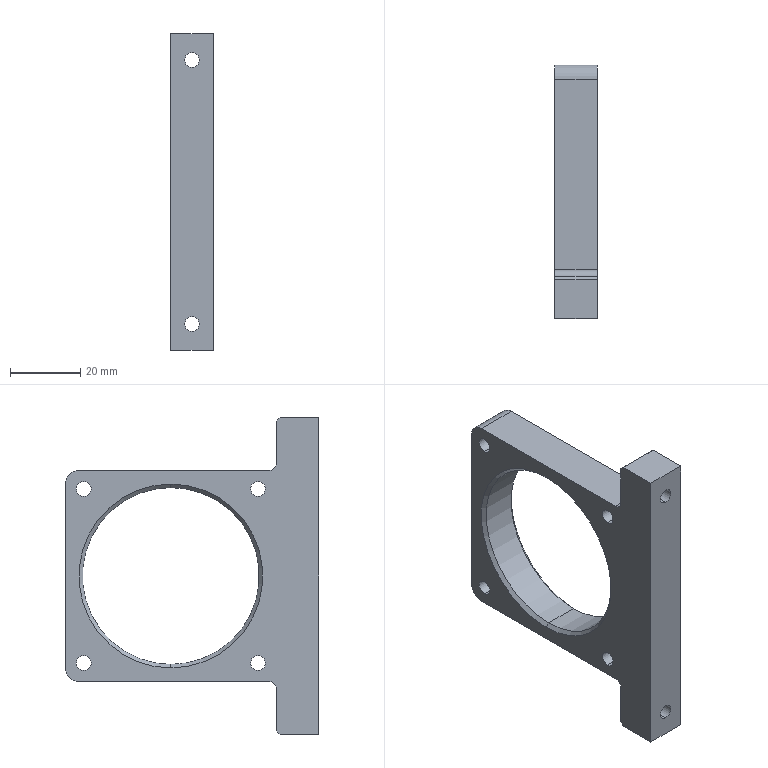Part | SolidWorks | features Chamfer 2, Fillet 2, HoleWzd 2, Extrusion 1 | 1 solid | 34 faces | box 12 x 72 x 90 mm | volume 31178 mm3 | cylinder 18 | plane 12 | cone 4 | commonest cylinder face diameters 4.2 x12 4 x2 8 x2 50.2 x2
STEP:
#1=CARTESIAN_POINT('',(5.,42.,25.1));
#2=VERTEX_POINT('',#1);
#3=CARTESIAN_POINT('',(5.,42.,-25.1));
#4=VERTEX_POINT('',#3);
#5=CARTESIAN_POINT('',(5.,42.,0.));
#6=DIRECTION('',(1.,0.,0.));
#7=DIRECTION('',(0.,0.,1.));
#8=AXIS2_PLACEMENT_3D('',#5,#6,#7);
#9=CIRCLE('',#8,25.1);
#10=EDGE_CURVE('',#2,#4,#9,.T.);
#11=ORIENTED_EDGE('',*,*,#10,.F.);
#12=CARTESIAN_POINT('',(6.,42.,26.1));
#13=VERTEX_POINT('',#12);
#14=CARTESIAN_POINT('',(5.,42.,25.1));
#15=DIRECTION('',(0.7071,0.,0.7071));
#16=VECTOR('',#15,1000.);
#17=LINE('',#14,#16);
#18=EDGE_CURVE('',#2,#13,#17,.T.);
#19=ORIENTED_EDGE('',*,*,#18,.T.);
#20=CARTESIAN_POINT('',(6.,42.,-26.1));
#21=VERTEX_POINT('',#20);
#22=CARTESIAN_POINT('',(6.,42.,0.));
#23=DIRECTION('',(-1.,0.,0.));
#24=DIRECTION('',(0.,0.,1.));
#25=AXIS2_PLACEMENT_3D('',#22,#23,#24);
#26=CIRCLE('',#25,26.1);
#27=EDGE_CURVE('',#21,#13,#26,.T.);
#28=ORIENTED_EDGE('',*,*,#27,.F.);
#29=CARTESIAN_POINT('',(5.,42.,-25.1));
#30=DIRECTION('',(0.7071,0.,-0.7071));
#31=VECTOR('',#30,1000.);
#32=LINE('',#29,#31);
#33=EDGE_CURVE('',#4,#21,#32,.T.);
#34=ORIENTED_EDGE('',*,*,#33,.F.);
#35=EDGE_LOOP('',(#11,#19,#28,#34));
#36=FACE_OUTER_BOUND('',#35,.T.);
#37=CARTESIAN_POINT('',(5.,42.,0.));
#38=DIRECTION('',(1.,0.,0.));
#39=DIRECTION('',(0.,0.,-1.));
#40=AXIS2_PLACEMENT_3D('',#37,#38,#39);
#41=CONICAL_SURFACE('',#40,25.1,0.7854);
#42=ADVANCED_FACE('',(#36),#41,.F.);
#43=CARTESIAN_POINT('',(-5.,42.,-25.1));
#44=VERTEX_POINT('',#43);
#45=CARTESIAN_POINT('',(-5.,42.,25.1));
#46=VERTEX_POINT('',#45);
#47=CARTESIAN_POINT('',(-5.,42.,0.));
#48=DIRECTION('',(-1.,0.,0.));
#49=DIRECTION('',(0.,0.,1.));
#50=AXIS2_PLACEMENT_3D('',#47,#48,#49);
#51=CIRCLE('',#50,25.1);
#52=EDGE_CURVE('',#44,#46,#51,.T.);
#53=ORIENTED_EDGE('',*,*,#52,.F.);
#54=CARTESIAN_POINT('',(-6.,42.,-26.1));
#55=VERTEX_POINT('',#54);
#56=CARTESIAN_POINT('',(-6.,42.,-26.1));
#57=DIRECTION('',(-0.7071,0.,-0.7071));
#58=VECTOR('',#57,1000.);
#59=LINE('',#56,#58);
#60=EDGE_CURVE('',#44,#55,#59,.T.);
#61=ORIENTED_EDGE('',*,*,#60,.T.);
#62=CARTESIAN_POINT('',(-6.,42.,26.1));
#63=VERTEX_POINT('',#62);
#64=CARTESIAN_POINT('',(-6.,42.,0.));
#65=DIRECTION('',(1.,0.,0.));
#66=DIRECTION('',(0.,0.,1.));
#67=AXIS2_PLACEMENT_3D('',#64,#65,#66);
#68=CIRCLE('',#67,26.1);
#69=EDGE_CURVE('',#63,#55,#68,.T.);
#70=ORIENTED_EDGE('',*,*,#69,.F.);
#71=CARTESIAN_POINT('',(-6.,42.,26.1));
#72=DIRECTION('',(-0.7071,0.,0.7071));
#73=VECTOR('',#72,1000.);
#74=LINE('',#71,#73);
#75=EDGE_CURVE('',#46,#63,#74,.T.);
#76=ORIENTED_EDGE('',*,*,#75,.F.);
#77=EDGE_LOOP('',(#53,#61,#70,#76));
#78=FACE_OUTER_BOUND('',#77,.T.);
#79=CARTESIAN_POINT('',(-6.,42.,0.));
#80=DIRECTION('',(-1.,0.,0.));
#81=DIRECTION('',(0.,0.,1.));
#82=AXIS2_PLACEMENT_3D('',#79,#80,#81);
#83=CONICAL_SURFACE('',#82,26.1,0.7854);
#84=ADVANCED_FACE('',(#78),#83,.F.);
#85=CARTESIAN_POINT('',(-6.,66.749,22.649));
#86=VERTEX_POINT('',#85);
#87=CARTESIAN_POINT('',(-6.,66.749,26.849));
#88=VERTEX_POINT('',#87);
#89=CARTESIAN_POINT('',(-6.,66.749,24.749));
#90=DIRECTION('',(-1.,0.,0.));
#91=DIRECTION('',(0.,0.,1.));
#92=AXIS2_PLACEMENT_3D('',#89,#90,#91);
#93=CIRCLE('',#92,2.1);
#94=EDGE_CURVE('',#86,#88,#93,.T.);
#95=ORIENTED_EDGE('',*,*,#94,.T.);
#96=CARTESIAN_POINT('',(6.,66.749,26.849));
#97=VERTEX_POINT('',#96);
#98=CARTESIAN_POINT('',(6.,66.749,26.849));
#99=DIRECTION('',(1.,0.,0.));
#100=VECTOR('',#99,1000.);
#101=LINE('',#98,#100);
#102=EDGE_CURVE('',#88,#97,#101,.T.);
#103=ORIENTED_EDGE('',*,*,#102,.T.);
#104=CARTESIAN_POINT('',(6.,66.749,22.649));
#105=VERTEX_POINT('',#104);
#106=CARTESIAN_POINT('',(6.,66.749,24.749));
#107=DIRECTION('',(1.,0.,0.));
#108=DIRECTION('',(0.,0.,-1.));
#109=AXIS2_PLACEMENT_3D('',#106,#107,#108);
#110=CIRCLE('',#109,2.1);
#111=EDGE_CURVE('',#97,#105,#110,.T.);
#112=ORIENTED_EDGE('',*,*,#111,.T.);
#113=CARTESIAN_POINT('',(6.,66.749,22.649));
#114=DIRECTION('',(1.,0.,0.));
#115=VECTOR('',#114,1000.);
#116=LINE('',#113,#115);
#117=EDGE_CURVE('',#86,#105,#116,.T.);
#118=ORIENTED_EDGE('',*,*,#117,.F.);
#119=EDGE_LOOP('',(#95,#103,#112,#118));
#120=FACE_OUTER_BOUND('',#119,.T.);
#121=CARTESIAN_POINT('',(6.,66.749,24.749));
#122=DIRECTION('',(1.,0.,0.));
#123=DIRECTION('',(0.,0.,-1.));
#124=AXIS2_PLACEMENT_3D('',#121,#122,#123);
#125=CYLINDRICAL_SURFACE('',#124,2.1);
#126=ADVANCED_FACE('',(#120),#125,.F.);
#127=CARTESIAN_POINT('',(-6.,66.749,-26.849));
#128=VERTEX_POINT('',#127);
#129=CARTESIAN_POINT('',(-6.,66.749,-22.649));
#130=VERTEX_POINT('',#129);
#131=CARTESIAN_POINT('',(-6.,66.749,-24.749));
#132=DIRECTION('',(-1.,0.,0.));
#133=DIRECTION('',(0.,0.,1.));
#134=AXIS2_PLACEMENT_3D('',#131,#132,#133);
#135=CIRCLE('',#134,2.1);
#136=EDGE_CURVE('',#128,#130,#135,.T.);
#137=ORIENTED_EDGE('',*,*,#136,.T.);
#138=CARTESIAN_POINT('',(6.,66.749,-22.649));
#139=VERTEX_POINT('',#138);
#140=CARTESIAN_POINT('',(6.,66.749,-22.649));
#141=DIRECTION('',(1.,0.,0.));
#142=VECTOR('',#141,1000.);
#143=LINE('',#140,#142);
#144=EDGE_CURVE('',#130,#139,#143,.T.);
#145=ORIENTED_EDGE('',*,*,#144,.T.);
#146=CARTESIAN_POINT('',(6.,66.749,-26.849));
#147=VERTEX_POINT('',#146);
#148=CARTESIAN_POINT('',(6.,66.749,-24.749));
#149=DIRECTION('',(1.,0.,0.));
#150=DIRECTION('',(0.,0.,-1.));
#151=AXIS2_PLACEMENT_3D('',#148,#149,#150);
#152=CIRCLE('',#151,2.1);
#153=EDGE_CURVE('',#139,#147,#152,.T.);
#154=ORIENTED_EDGE('',*,*,#153,.T.);
#155=CARTESIAN_POINT('',(6.,66.749,-26.849));
#156=DIRECTION('',(1.,0.,0.));
#157=VECTOR('',#156,1000.);
#158=LINE('',#155,#157);
#159=EDGE_CURVE('',#128,#147,#158,.T.);
#160=ORIENTED_EDGE('',*,*,#159,.F.);
#161=EDGE_LOOP('',(#137,#145,#154,#160));
#162=FACE_OUTER_BOUND('',#161,.T.);
#163=CARTESIAN_POINT('',(6.,66.749,-24.749));
#164=DIRECTION('',(1.,0.,0.));
#165=DIRECTION('',(0.,0.,-1.));
#166=AXIS2_PLACEMENT_3D('',#163,#164,#165);
#167=CYLINDRICAL_SURFACE('',#166,2.1);
#168=ADVANCED_FACE('',(#162),#167,.F.);
#169=CARTESIAN_POINT('',(-6.,17.251,-26.849));
#170=VERTEX_POINT('',#169);
#171=CARTESIAN_POINT('',(-6.,17.251,-22.649));
#172=VERTEX_POINT('',#171);
#173=CARTESIAN_POINT('',(-6.,17.251,-24.749));
#174=DIRECTION('',(-1.,0.,0.));
#175=DIRECTION('',(0.,0.,1.));
#176=AXIS2_PLACEMENT_3D('',#173,#174,#175);
#177=CIRCLE('',#176,2.1);
#178=EDGE_CURVE('',#170,#172,#177,.T.);
#179=ORIENTED_EDGE('',*,*,#178,.T.);
#180=CARTESIAN_POINT('',(6.,17.251,-22.649));
#181=VERTEX_POINT('',#180);
#182=CARTESIAN_POINT('',(6.,17.251,-22.649));
#183=DIRECTION('',(1.,0.,0.));
#184=VECTOR('',#183,1000.);
#185=LINE('',#182,#184);
#186=EDGE_CURVE('',#172,#181,#185,.T.);
#187=ORIENTED_EDGE('',*,*,#186,.T.);
#188=CARTESIAN_POINT('',(6.,17.251,-26.849));
#189=VERTEX_POINT('',#188);
#190=CARTESIAN_POINT('',(6.,17.251,-24.749));
#191=DIRECTION('',(1.,0.,0.));
#192=DIRECTION('',(0.,0.,-1.));
#193=AXIS2_PLACEMENT_3D('',#190,#191,#192);
#194=CIRCLE('',#193,2.1);
#195=EDGE_CURVE('',#181,#189,#194,.T.);
#196=ORIENTED_EDGE('',*,*,#195,.T.);
#197=CARTESIAN_POINT('',(6.,17.251,-26.849));
#198=DIRECTION('',(1.,0.,0.));
#199=VECTOR('',#198,1000.);
#200=LINE('',#197,#199);
#201=EDGE_CURVE('',#170,#189,#200,.T.);
#202=ORIENTED_EDGE('',*,*,#201,.F.);
#203=EDGE_LOOP('',(#179,#187,#196,#202));
#204=FACE_OUTER_BOUND('',#203,.T.);
#205=CARTESIAN_POINT('',(6.,17.251,-24.749));
#206=DIRECTION('',(1.,0.,0.));
#207=DIRECTION('',(0.,0.,-1.));
#208=AXIS2_PLACEMENT_3D('',#205,#206,#207);
#209=CYLINDRICAL_SURFACE('',#208,2.1);
#210=ADVANCED_FACE('',(#204),#209,.F.);
#211=CARTESIAN_POINT('',(-6.,17.251,22.649));
#212=VERTEX_POINT('',#211);
#213=CARTESIAN_POINT('',(-6.,17.251,26.849));
#214=VERTEX_POINT('',#213);
#215=CARTESIAN_POINT('',(-6.,17.251,24.749));
#216=DIRECTION('',(-1.,0.,0.));
#217=DIRECTION('',(0.,0.,1.));
#218=AXIS2_PLACEMENT_3D('',#215,#216,#217);
#219=CIRCLE('',#218,2.1);
#220=EDGE_CURVE('',#212,#214,#219,.T.);
#221=ORIENTED_EDGE('',*,*,#220,.T.);
#222=CARTESIAN_POINT('',(6.,17.251,26.849));
#223=VERTEX_POINT('',#222);
#224=CARTESIAN_POINT('',(6.,17.251,26.849));
#225=DIRECTION('',(1.,0.,0.));
#226=VECTOR('',#225,1000.);
#227=LINE('',#224,#226);
#228=EDGE_CURVE('',#214,#223,#227,.T.);
#229=ORIENTED_EDGE('',*,*,#228,.T.);
#230=CARTESIAN_POINT('',(6.,17.251,22.649));
#231=VERTEX_POINT('',#230);
#232=CARTESIAN_POINT('',(6.,17.251,24.749));
#233=DIRECTION('',(1.,0.,0.));
#234=DIRECTION('',(0.,0.,-1.));
#235=AXIS2_PLACEMENT_3D('',#232,#233,#234);
#236=CIRCLE('',#235,2.1);
#237=EDGE_CURVE('',#223,#231,#236,.T.);
#238=ORIENTED_EDGE('',*,*,#237,.T.);
#239=CARTESIAN_POINT('',(6.,17.251,22.649));
#240=DIRECTION('',(1.,0.,0.));
#241=VECTOR('',#240,1000.);
#242=LINE('',#239,#241);
#243=EDGE_CURVE('',#212,#231,#242,.T.);
#244=ORIENTED_EDGE('',*,*,#243,.F.);
#245=EDGE_LOOP('',(#221,#229,#238,#244));
#246=FACE_OUTER_BOUND('',#245,.T.);
#247=CARTESIAN_POINT('',(6.,17.251,24.749));
#248=DIRECTION('',(1.,0.,0.));
#249=DIRECTION('',(0.,0.,-1.));
#250=AXIS2_PLACEMENT_3D('',#247,#248,#249);
#251=CYLINDRICAL_SURFACE('',#250,2.1);
#252=ADVANCED_FACE('',(#246),#251,.F.);
#253=CARTESIAN_POINT('',(0.,0.,35.4));
#254=VERTEX_POINT('',#253);
#255=CARTESIAN_POINT('',(0.,0.,39.6));
#256=VERTEX_POINT('',#255);
#257=CARTESIAN_POINT('',(0.,0.,37.5));
#258=DIRECTION('',(0.,1.,0.));
#259=DIRECTION('',(0.,0.,1.));
#260=AXIS2_PLACEMENT_3D('',#257,#258,#259);
#261=CIRCLE('',#260,2.1);
#262=EDGE_CURVE('',#254,#256,#261,.T.);
#263=ORIENTED_EDGE('',*,*,#262,.F.);
#264=CARTESIAN_POINT('',(0.,12.,35.4));
#265=VERTEX_POINT('',#264);
#266=CARTESIAN_POINT('',(0.,12.,35.4));
#267=DIRECTION('',(0.,1.,0.));
#268=VECTOR('',#267,1000.);
#269=LINE('',#266,#268);
#270=EDGE_CURVE('',#254,#265,#269,.T.);
#271=ORIENTED_EDGE('',*,*,#270,.T.);
#272=CARTESIAN_POINT('',(0.,12.,39.6));
#273=VERTEX_POINT('',#272);
#274=CARTESIAN_POINT('',(0.,12.,37.5));
#275=DIRECTION('',(0.,1.,0.));
#276=DIRECTION('',(0.,0.,1.));
#277=AXIS2_PLACEMENT_3D('',#274,#275,#276);
#278=CIRCLE('',#277,2.1);
#279=EDGE_CURVE('',#265,#273,#278,.T.);
#280=ORIENTED_EDGE('',*,*,#279,.T.);
#281=CARTESIAN_POINT('',(0.,12.,39.6));
#282=DIRECTION('',(0.,1.,0.));
#283=VECTOR('',#282,1000.);
#284=LINE('',#281,#283);
#285=EDGE_CURVE('',#256,#273,#284,.T.);
#286=ORIENTED_EDGE('',*,*,#285,.F.);
#287=EDGE_LOOP('',(#263,#271,#280,#286));
#288=FACE_OUTER_BOUND('',#287,.T.);
#289=CARTESIAN_POINT('',(0.,12.,37.5));
#290=DIRECTION('',(0.,1.,0.));
#291=DIRECTION('',(0.,0.,1.));
#292=AXIS2_PLACEMENT_3D('',#289,#290,#291);
#293=CYLINDRICAL_SURFACE('',#292,2.1);
#294=ADVANCED_FACE('',(#288),#293,.F.);
#295=CARTESIAN_POINT('',(0.,0.,-39.6));
#296=VERTEX_POINT('',#295);
#297=CARTESIAN_POINT('',(0.,0.,-35.4));
#298=VERTEX_POINT('',#297);
#299=CARTESIAN_POINT('',(0.,0.,-37.5));
#300=DIRECTION('',(0.,1.,0.));
#301=DIRECTION('',(0.,0.,1.));
#302=AXIS2_PLACEMENT_3D('',#299,#300,#301);
#303=CIRCLE('',#302,2.1);
#304=EDGE_CURVE('',#296,#298,#303,.T.);
#305=ORIENTED_EDGE('',*,*,#304,.F.);
#306=CARTESIAN_POINT('',(0.,12.,-39.6));
#307=VERTEX_POINT('',#306);
#308=CARTESIAN_POINT('',(0.,12.,-39.6));
#309=DIRECTION('',(0.,1.,0.));
#310=VECTOR('',#309,1000.);
#311=LINE('',#308,#310);
#312=EDGE_CURVE('',#296,#307,#311,.T.);
#313=ORIENTED_EDGE('',*,*,#312,.T.);
#314=CARTESIAN_POINT('',(0.,12.,-35.4));
#315=VERTEX_POINT('',#314);
#316=CARTESIAN_POINT('',(0.,12.,-37.5));
#317=DIRECTION('',(0.,1.,0.));
#318=DIRECTION('',(0.,0.,1.));
#319=AXIS2_PLACEMENT_3D('',#316,#317,#318);
#320=CIRCLE('',#319,2.1);
#321=EDGE_CURVE('',#307,#315,#320,.T.);
#322=ORIENTED_EDGE('',*,*,#321,.T.);
#323=CARTESIAN_POINT('',(0.,12.,-35.4));
#324=DIRECTION('',(0.,1.,0.));
#325=VECTOR('',#324,1000.);
#326=LINE('',#323,#325);
#327=EDGE_CURVE('',#298,#315,#326,.T.);
#328=ORIENTED_EDGE('',*,*,#327,.F.);
#329=EDGE_LOOP('',(#305,#313,#322,#328));
#330=FACE_OUTER_BOUND('',#329,.T.);
#331=CARTESIAN_POINT('',(0.,12.,-37.5));
#332=DIRECTION('',(0.,1.,0.));
#333=DIRECTION('',(0.,0.,1.));
#334=AXIS2_PLACEMENT_3D('',#331,#332,#333);
#335=CYLINDRICAL_SURFACE('',#334,2.1);
#336=ADVANCED_FACE('',(#330),#335,.F.);
#337=ORIENTED_EDGE('',*,*,#10,.T.);
#338=CARTESIAN_POINT('',(6.,42.,-25.1));
#339=DIRECTION('',(-1.,0.,0.));
#340=VECTOR('',#339,1000.);
#341=LINE('',#338,#340);
#342=EDGE_CURVE('',#4,#44,#341,.T.);
#343=ORIENTED_EDGE('',*,*,#342,.T.);
#344=ORIENTED_EDGE('',*,*,#52,.T.);
#345=CARTESIAN_POINT('',(6.,42.,25.1));
#346=DIRECTION('',(-1.,0.,0.));
#347=VECTOR('',#346,1000.);
#348=LINE('',#345,#347);
#349=EDGE_CURVE('',#2,#46,#348,.T.);
#350=ORIENTED_EDGE('',*,*,#349,.F.);
#351=EDGE_LOOP('',(#337,#343,#344,#350));
#352=FACE_OUTER_BOUND('',#351,.T.);
#353=CARTESIAN_POINT('',(6.,42.,0.));
#354=DIRECTION('',(-1.,0.,0.));
#355=DIRECTION('',(0.,0.,1.));
#356=AXIS2_PLACEMENT_3D('',#353,#354,#355);
#357=CYLINDRICAL_SURFACE('',#356,25.1);
#358=ADVANCED_FACE('',(#352),#357,.F.);
#359=ORIENTED_EDGE('',*,*,#27,.T.);
#360=CARTESIAN_POINT('',(6.,42.,0.));
#361=DIRECTION('',(-1.,0.,0.));
#362=DIRECTION('',(0.,0.,1.));
#363=AXIS2_PLACEMENT_3D('',#360,#361,#362);
#364=CIRCLE('',#363,26.1);
#365=EDGE_CURVE('',#13,#21,#364,.T.);
#366=ORIENTED_EDGE('',*,*,#365,.T.);
#367=EDGE_LOOP('',(#359,#366));
#368=FACE_BOUND('',#367,.T.);
#369=CARTESIAN_POINT('',(6.,66.749,24.749));
#370=DIRECTION('',(1.,0.,0.));
#371=DIRECTION('',(0.,0.,-1.));
#372=AXIS2_PLACEMENT_3D('',#369,#370,#371);
#373=CIRCLE('',#372,2.1);
#374=EDGE_CURVE('',#105,#97,#373,.T.);
#375=ORIENTED_EDGE('',*,*,#374,.F.);
#376=ORIENTED_EDGE('',*,*,#111,.F.);
#377=EDGE_LOOP('',(#375,#376));
#378=FACE_BOUND('',#377,.T.);
#379=CARTESIAN_POINT('',(6.,66.749,-24.749));
#380=DIRECTION('',(1.,0.,0.));
#381=DIRECTION('',(0.,0.,-1.));
#382=AXIS2_PLACEMENT_3D('',#379,#380,#381);
#383=CIRCLE('',#382,2.1);
#384=EDGE_CURVE('',#147,#139,#383,.T.);
#385=ORIENTED_EDGE('',*,*,#384,.F.);
#386=ORIENTED_EDGE('',*,*,#153,.F.);
#387=EDGE_LOOP('',(#385,#386));
#388=FACE_BOUND('',#387,.T.);
#389=CARTESIAN_POINT('',(6.,17.251,-24.749));
#390=DIRECTION('',(1.,0.,0.));
#391=DIRECTION('',(0.,0.,-1.));
#392=AXIS2_PLACEMENT_3D('',#389,#390,#391);
#393=CIRCLE('',#392,2.1);
#394=EDGE_CURVE('',#189,#181,#393,.T.);
#395=ORIENTED_EDGE('',*,*,#394,.F.);
#396=ORIENTED_EDGE('',*,*,#195,.F.);
#397=EDGE_LOOP('',(#395,#396));
#398=FACE_BOUND('',#397,.T.);
#399=CARTESIAN_POINT('',(6.,17.251,24.749));
#400=DIRECTION('',(1.,0.,0.));
#401=DIRECTION('',(0.,0.,-1.));
#402=AXIS2_PLACEMENT_3D('',#399,#400,#401);
#403=CIRCLE('',#402,2.1);
#404=EDGE_CURVE('',#231,#223,#403,.T.);
#405=ORIENTED_EDGE('',*,*,#404,.F.);
#406=ORIENTED_EDGE('',*,*,#237,.F.);
#407=EDGE_LOOP('',(#405,#406));
#408=FACE_BOUND('',#407,.T.);
#409=CARTESIAN_POINT('',(6.,12.,32.));
#410=VERTEX_POINT('',#409);
#411=CARTESIAN_POINT('',(6.,12.,44.));
#412=VERTEX_POINT('',#411);
#413=CARTESIAN_POINT('',(6.,12.,45.));
#414=DIRECTION('',(0.,0.,1.));
#415=VECTOR('',#414,1000.);
#416=LINE('',#413,#415);
#417=EDGE_CURVE('',#410,#412,#416,.T.);
#418=ORIENTED_EDGE('',*,*,#417,.T.);
#419=CARTESIAN_POINT('',(6.,11.,45.));
#420=VERTEX_POINT('',#419);
#421=CARTESIAN_POINT('',(6.,11.,45.));
#422=DIRECTION('',(0.,-0.7071,0.7071));
#423=VECTOR('',#422,1000.);
#424=LINE('',#421,#423);
#425=EDGE_CURVE('',#412,#420,#424,.T.);
#426=ORIENTED_EDGE('',*,*,#425,.T.);
#427=CARTESIAN_POINT('',(6.,0.,45.));
#428=VERTEX_POINT('',#427);
#429=CARTESIAN_POINT('',(6.,0.,45.));
#430=DIRECTION('',(0.,-1.,0.));
#431=VECTOR('',#430,1000.);
#432=LINE('',#429,#431);
#433=EDGE_CURVE('',#420,#428,#432,.T.);
#434=ORIENTED_EDGE('',*,*,#433,.T.);
#435=CARTESIAN_POINT('',(6.,0.,-45.));
#436=VERTEX_POINT('',#435);
#437=CARTESIAN_POINT('',(6.,0.,45.));
#438=DIRECTION('',(0.,0.,-1.));
#439=VECTOR('',#438,1000.);
#440=LINE('',#437,#439);
#441=EDGE_CURVE('',#428,#436,#440,.T.);
#442=ORIENTED_EDGE('',*,*,#441,.T.);
#443=CARTESIAN_POINT('',(6.,11.,-45.));
#444=VERTEX_POINT('',#443);
#445=CARTESIAN_POINT('',(6.,0.,-45.));
#446=DIRECTION('',(0.,1.,0.));
#447=VECTOR('',#446,1000.);
#448=LINE('',#445,#447);
#449=EDGE_CURVE('',#436,#444,#448,.T.);
#450=ORIENTED_EDGE('',*,*,#449,.T.);
#451=CARTESIAN_POINT('',(6.,12.,-44.));
#452=VERTEX_POINT('',#451);
#453=CARTESIAN_POINT('',(6.,12.,-44.));
#454=DIRECTION('',(0.,0.7071,0.7071));
#455=VECTOR('',#454,1000.);
#456=LINE('',#453,#455);
#457=EDGE_CURVE('',#444,#452,#456,.T.);
#458=ORIENTED_EDGE('',*,*,#457,.T.);
#459=CARTESIAN_POINT('',(6.,12.,-32.));
#460=VERTEX_POINT('',#459);
#461=CARTESIAN_POINT('',(6.,12.,-45.));
#462=DIRECTION('',(0.,0.,1.));
#463=VECTOR('',#462,1000.);
#464=LINE('',#461,#463);
#465=EDGE_CURVE('',#452,#460,#464,.T.);
#466=ORIENTED_EDGE('',*,*,#465,.T.);
#467=CARTESIAN_POINT('',(6.,14.,-30.));
#468=VERTEX_POINT('',#467);
#469=CARTESIAN_POINT('',(6.,14.,-32.));
#470=DIRECTION('',(-1.,0.,0.));
#471=DIRECTION('',(0.,0.,1.));
#472=AXIS2_PLACEMENT_3D('',#469,#470,#471);
#473=CIRCLE('',#472,2.);
#474=EDGE_CURVE('',#460,#468,#473,.T.);
#475=ORIENTED_EDGE('',*,*,#474,.T.);
#476=CARTESIAN_POINT('',(6.,68.,-30.));
#477=VERTEX_POINT('',#476);
#478=CARTESIAN_POINT('',(6.,72.,-30.));
#479=DIRECTION('',(0.,1.,0.));
#480=VECTOR('',#479,1000.);
#481=LINE('',#478,#480);
#482=EDGE_CURVE('',#468,#477,#481,.T.);
#483=ORIENTED_EDGE('',*,*,#482,.T.);
#484=CARTESIAN_POINT('',(6.,72.,-26.));
#485=VERTEX_POINT('',#484);
#486=CARTESIAN_POINT('',(6.,68.,-26.));
#487=DIRECTION('',(1.,0.,0.));
#488=DIRECTION('',(0.,0.,1.));
#489=AXIS2_PLACEMENT_3D('',#486,#487,#488);
#490=CIRCLE('',#489,4.);
#491=EDGE_CURVE('',#477,#485,#490,.T.);
#492=ORIENTED_EDGE('',*,*,#491,.T.);
#493=CARTESIAN_POINT('',(6.,72.,26.));
#494=VERTEX_POINT('',#493);
#495=CARTESIAN_POINT('',(6.,72.,30.));
#496=DIRECTION('',(0.,0.,1.));
#497=VECTOR('',#496,1000.);
#498=LINE('',#495,#497);
#499=EDGE_CURVE('',#485,#494,#498,.T.);
#500=ORIENTED_EDGE('',*,*,#499,.T.);
#501=CARTESIAN_POINT('',(6.,68.,30.));
#502=VERTEX_POINT('',#501);
#503=CARTESIAN_POINT('',(6.,68.,26.));
#504=DIRECTION('',(1.,0.,0.));
#505=DIRECTION('',(0.,0.,1.));
#506=AXIS2_PLACEMENT_3D('',#503,#504,#505);
#507=CIRCLE('',#506,4.);
#508=EDGE_CURVE('',#494,#502,#507,.T.);
#509=ORIENTED_EDGE('',*,*,#508,.T.);
#510=CARTESIAN_POINT('',(6.,14.,30.));
#511=VERTEX_POINT('',#510);
#512=CARTESIAN_POINT('',(6.,72.,30.));
#513=DIRECTION('',(0.,-1.,0.));
#514=VECTOR('',#513,1000.);
#515=LINE('',#512,#514);
#516=EDGE_CURVE('',#502,#511,#515,.T.);
#517=ORIENTED_EDGE('',*,*,#516,.T.);
#518=CARTESIAN_POINT('',(6.,14.,32.));
#519=DIRECTION('',(-1.,0.,0.));
#520=DIRECTION('',(0.,0.,1.));
#521=AXIS2_PLACEMENT_3D('',#518,#519,#520);
#522=CIRCLE('',#521,2.);
#523=EDGE_CURVE('',#511,#410,#522,.T.);
#524=ORIENTED_EDGE('',*,*,#523,.T.);
#525=EDGE_LOOP('',(#418,#426,#434,#442,#450,#458,#466,#475,#483,#492,#500,#509,#517,#524));
#526=FACE_OUTER_BOUND('',#525,.T.);
#527=CARTESIAN_POINT('',(6.,0.,0.));
#528=DIRECTION('',(-1.,0.,0.));
#529=DIRECTION('',(0.,0.,1.));
#530=AXIS2_PLACEMENT_3D('',#527,#528,#529);
#531=PLANE('',#530);
#532=ADVANCED_FACE('',(#368,#378,#388,#398,#408,#526),#531,.F.);
#533=ORIENTED_EDGE('',*,*,#69,.T.);
#534=CARTESIAN_POINT('',(-6.,42.,0.));
#535=DIRECTION('',(1.,0.,0.));
#536=DIRECTION('',(0.,0.,1.));
#537=AXIS2_PLACEMENT_3D('',#534,#535,#536);
#538=CIRCLE('',#537,26.1);
#539=EDGE_CURVE('',#55,#63,#538,.T.);
#540=ORIENTED_EDGE('',*,*,#539,.T.);
#541=EDGE_LOOP('',(#533,#540));
#542=FACE_BOUND('',#541,.T.);
#543=ORIENTED_EDGE('',*,*,#94,.F.);
#544=CARTESIAN_POINT('',(-6.,66.749,24.749));
#545=DIRECTION('',(-1.,0.,0.));
#546=DIRECTION('',(0.,0.,1.));
#547=AXIS2_PLACEMENT_3D('',#544,#545,#546);
#548=CIRCLE('',#547,2.1);
#549=EDGE_CURVE('',#88,#86,#548,.T.);
#550=ORIENTED_EDGE('',*,*,#549,.F.);
#551=EDGE_LOOP('',(#543,#550));
#552=FACE_BOUND('',#551,.T.);
#553=ORIENTED_EDGE('',*,*,#136,.F.);
#554=CARTESIAN_POINT('',(-6.,66.749,-24.749));
#555=DIRECTION('',(-1.,0.,0.));
#556=DIRECTION('',(0.,0.,1.));
#557=AXIS2_PLACEMENT_3D('',#554,#555,#556);
#558=CIRCLE('',#557,2.1);
#559=EDGE_CURVE('',#130,#128,#558,.T.);
#560=ORIENTED_EDGE('',*,*,#559,.F.);
#561=EDGE_LOOP('',(#553,#560));
#562=FACE_BOUND('',#561,.T.);
#563=ORIENTED_EDGE('',*,*,#178,.F.);
#564=CARTESIAN_POINT('',(-6.,17.251,-24.749));
#565=DIRECTION('',(-1.,0.,0.));
#566=DIRECTION('',(0.,0.,1.));
#567=AXIS2_PLACEMENT_3D('',#564,#565,#566);
#568=CIRCLE('',#567,2.1);
#569=EDGE_CURVE('',#172,#170,#568,.T.);
#570=ORIENTED_EDGE('',*,*,#569,.F.);
#571=EDGE_LOOP('',(#563,#570));
#572=FACE_BOUND('',#571,.T.);
#573=ORIENTED_EDGE('',*,*,#220,.F.);
#574=CARTESIAN_POINT('',(-6.,17.251,24.749));
#575=DIRECTION('',(-1.,0.,0.));
#576=DIRECTION('',(0.,0.,1.));
#577=AXIS2_PLACEMENT_3D('',#574,#575,#576);
#578=CIRCLE('',#577,2.1);
#579=EDGE_CURVE('',#214,#212,#578,.T.);
#580=ORIENTED_EDGE('',*,*,#579,.F.);
#581=EDGE_LOOP('',(#573,#580));
#582=FACE_BOUND('',#581,.T.);
#583=CARTESIAN_POINT('',(-6.,11.,45.));
#584=VERTEX_POINT('',#583);
#585=CARTESIAN_POINT('',(-6.,0.,45.));
#586=VERTEX_POINT('',#585);
#587=CARTESIAN_POINT('',(-6.,0.,45.));
#588=DIRECTION('',(0.,-1.,0.));
#589=VECTOR('',#588,1000.);
#590=LINE('',#587,#589);
#591=EDGE_CURVE('',#584,#586,#590,.T.);
#592=ORIENTED_EDGE('',*,*,#591,.F.);
#593=CARTESIAN_POINT('',(-6.,12.,44.));
#594=VERTEX_POINT('',#593);
#595=CARTESIAN_POINT('',(-6.,28.,28.));
#596=DIRECTION('',(0.,0.7071,-0.7071));
#597=VECTOR('',#596,1000.);
#598=LINE('',#595,#597);
#599=EDGE_CURVE('',#584,#594,#598,.T.);
#600=ORIENTED_EDGE('',*,*,#599,.T.);
#601=CARTESIAN_POINT('',(-6.,12.,32.));
#602=VERTEX_POINT('',#601);
#603=CARTESIAN_POINT('',(-6.,12.,45.));
#604=DIRECTION('',(0.,0.,1.));
#605=VECTOR('',#604,1000.);
#606=LINE('',#603,#605);
#607=EDGE_CURVE('',#602,#594,#606,.T.);
#608=ORIENTED_EDGE('',*,*,#607,.F.);
#609=CARTESIAN_POINT('',(-6.,14.,30.));
#610=VERTEX_POINT('',#609);
#611=CARTESIAN_POINT('',(-6.,14.,32.));
#612=DIRECTION('',(1.,0.,0.));
#613=DIRECTION('',(0.,0.,1.));
#614=AXIS2_PLACEMENT_3D('',#611,#612,#613);
#615=CIRCLE('',#614,2.);
#616=EDGE_CURVE('',#602,#610,#615,.T.);
#617=ORIENTED_EDGE('',*,*,#616,.T.);
#618=CARTESIAN_POINT('',(-6.,68.,30.));
#619=VERTEX_POINT('',#618);
#620=CARTESIAN_POINT('',(-6.,72.,30.));
#621=DIRECTION('',(0.,-1.,0.));
#622=VECTOR('',#621,1000.);
#623=LINE('',#620,#622);
#624=EDGE_CURVE('',#619,#610,#623,.T.);
#625=ORIENTED_EDGE('',*,*,#624,.F.);
#626=CARTESIAN_POINT('',(-6.,72.,26.));
#627=VERTEX_POINT('',#626);
#628=CARTESIAN_POINT('',(-6.,68.,26.));
#629=DIRECTION('',(-1.,0.,0.));
#630=DIRECTION('',(0.,0.,1.));
#631=AXIS2_PLACEMENT_3D('',#628,#629,#630);
#632=CIRCLE('',#631,4.);
#633=EDGE_CURVE('',#619,#627,#632,.T.);
#634=ORIENTED_EDGE('',*,*,#633,.T.);
#635=CARTESIAN_POINT('',(-6.,72.,-26.));
#636=VERTEX_POINT('',#635);
#637=CARTESIAN_POINT('',(-6.,72.,30.));
#638=DIRECTION('',(0.,0.,1.));
#639=VECTOR('',#638,1000.);
#640=LINE('',#637,#639);
#641=EDGE_CURVE('',#636,#627,#640,.T.);
#642=ORIENTED_EDGE('',*,*,#641,.F.);
#643=CARTESIAN_POINT('',(-6.,68.,-30.));
#644=VERTEX_POINT('',#643);
#645=CARTESIAN_POINT('',(-6.,68.,-26.));
#646=DIRECTION('',(-1.,0.,0.));
#647=DIRECTION('',(0.,0.,1.));
#648=AXIS2_PLACEMENT_3D('',#645,#646,#647);
#649=CIRCLE('',#648,4.);
#650=EDGE_CURVE('',#636,#644,#649,.T.);
#651=ORIENTED_EDGE('',*,*,#650,.T.);
#652=CARTESIAN_POINT('',(-6.,14.,-30.));
#653=VERTEX_POINT('',#652);
#654=CARTESIAN_POINT('',(-6.,72.,-30.));
#655=DIRECTION('',(0.,1.,0.));
#656=VECTOR('',#655,1000.);
#657=LINE('',#654,#656);
#658=EDGE_CURVE('',#653,#644,#657,.T.);
#659=ORIENTED_EDGE('',*,*,#658,.F.);
#660=CARTESIAN_POINT('',(-6.,12.,-32.));
#661=VERTEX_POINT('',#660);
#662=CARTESIAN_POINT('',(-6.,14.,-32.));
#663=DIRECTION('',(1.,0.,0.));
#664=DIRECTION('',(0.,0.,1.));
#665=AXIS2_PLACEMENT_3D('',#662,#663,#664);
#666=CIRCLE('',#665,2.);
#667=EDGE_CURVE('',#653,#661,#666,.T.);
#668=ORIENTED_EDGE('',*,*,#667,.T.);
#669=CARTESIAN_POINT('',(-6.,12.,-44.));
#670=VERTEX_POINT('',#669);
#671=CARTESIAN_POINT('',(-6.,12.,-45.));
#672=DIRECTION('',(0.,0.,1.));
#673=VECTOR('',#672,1000.);
#674=LINE('',#671,#673);
#675=EDGE_CURVE('',#670,#661,#674,.T.);
#676=ORIENTED_EDGE('',*,*,#675,.F.);
#677=CARTESIAN_POINT('',(-6.,11.,-45.));
#678=VERTEX_POINT('',#677);
#679=CARTESIAN_POINT('',(-6.,28.,-28.));
#680=DIRECTION('',(0.,-0.7071,-0.7071));
#681=VECTOR('',#680,1000.);
#682=LINE('',#679,#681);
#683=EDGE_CURVE('',#670,#678,#682,.T.);
#684=ORIENTED_EDGE('',*,*,#683,.T.);
#685=CARTESIAN_POINT('',(-6.,0.,-45.));
#686=VERTEX_POINT('',#685);
#687=CARTESIAN_POINT('',(-6.,0.,-45.));
#688=DIRECTION('',(0.,1.,0.));
#689=VECTOR('',#688,1000.);
#690=LINE('',#687,#689);
#691=EDGE_CURVE('',#686,#678,#690,.T.);
#692=ORIENTED_EDGE('',*,*,#691,.F.);
#693=CARTESIAN_POINT('',(-6.,0.,45.));
#694=DIRECTION('',(0.,0.,-1.));
#695=VECTOR('',#694,1000.);
#696=LINE('',#693,#695);
#697=EDGE_CURVE('',#586,#686,#696,.T.);
#698=ORIENTED_EDGE('',*,*,#697,.F.);
#699=EDGE_LOOP('',(#592,#600,#608,#617,#625,#634,#642,#651,#659,#668,#676,#684,#692,#698));
#700=FACE_OUTER_BOUND('',#699,.T.);
#701=CARTESIAN_POINT('',(-6.,0.,0.));
#702=DIRECTION('',(-1.,0.,0.));
#703=DIRECTION('',(0.,0.,1.));
#704=AXIS2_PLACEMENT_3D('',#701,#702,#703);
#705=PLANE('',#704);
#706=ADVANCED_FACE('',(#542,#552,#562,#572,#582,#700),#705,.T.);
#707=ORIENTED_EDGE('',*,*,#433,.F.);
#708=CARTESIAN_POINT('',(6.,11.,45.));
#709=DIRECTION('',(-1.,0.,0.));
#710=VECTOR('',#709,1000.);
#711=LINE('',#708,#710);
#712=EDGE_CURVE('',#420,#584,#711,.T.);
#713=ORIENTED_EDGE('',*,*,#712,.T.);
#714=ORIENTED_EDGE('',*,*,#591,.T.);
#715=CARTESIAN_POINT('',(6.,0.,45.));
#716=DIRECTION('',(-1.,0.,0.));
#717=VECTOR('',#716,1000.);
#718=LINE('',#715,#717);
#719=EDGE_CURVE('',#428,#586,#718,.T.);
#720=ORIENTED_EDGE('',*,*,#719,.F.);
#721=EDGE_LOOP('',(#707,#713,#714,#720));
#722=FACE_OUTER_BOUND('',#721,.T.);
#723=CARTESIAN_POINT('',(6.,0.,45.));
#724=DIRECTION('',(0.,0.,-1.));
#725=DIRECTION('',(0.,1.,0.));
#726=AXIS2_PLACEMENT_3D('',#723,#724,#725);
#727=PLANE('',#726);
#728=ADVANCED_FACE('',(#722),#727,.F.);
#729=CARTESIAN_POINT('',(0.,0.,37.5));
#730=DIRECTION('',(0.,1.,0.));
#731=DIRECTION('',(0.,0.,1.));
#732=AXIS2_PLACEMENT_3D('',#729,#730,#731);
#733=CIRCLE('',#732,2.1);
#734=EDGE_CURVE('',#256,#254,#733,.T.);
#735=ORIENTED_EDGE('',*,*,#734,.T.);
#736=ORIENTED_EDGE('',*,*,#262,.T.);
#737=EDGE_LOOP('',(#735,#736));
#738=FACE_BOUND('',#737,.T.);
#739=CARTESIAN_POINT('',(0.,0.,-37.5));
#740=DIRECTION('',(0.,1.,0.));
#741=DIRECTION('',(0.,0.,1.));
#742=AXIS2_PLACEMENT_3D('',#739,#740,#741);
#743=CIRCLE('',#742,2.1);
#744=EDGE_CURVE('',#298,#296,#743,.T.);
#745=ORIENTED_EDGE('',*,*,#744,.T.);
#746=ORIENTED_EDGE('',*,*,#304,.T.);
#747=EDGE_LOOP('',(#745,#746));
#748=FACE_BOUND('',#747,.T.);
#749=ORIENTED_EDGE('',*,*,#697,.T.);
#750=CARTESIAN_POINT('',(6.,0.,-45.));
#751=DIRECTION('',(-1.,0.,0.));
#752=VECTOR('',#751,1000.);
#753=LINE('',#750,#752);
#754=EDGE_CURVE('',#436,#686,#753,.T.);
#755=ORIENTED_EDGE('',*,*,#754,.F.);
#756=ORIENTED_EDGE('',*,*,#441,.F.);
#757=ORIENTED_EDGE('',*,*,#719,.T.);
#758=EDGE_LOOP('',(#749,#755,#756,#757));
#759=FACE_OUTER_BOUND('',#758,.T.);
#760=CARTESIAN_POINT('',(6.,0.,45.));
#761=DIRECTION('',(0.,1.,0.));
#762=DIRECTION('',(0.,0.,1.));
#763=AXIS2_PLACEMENT_3D('',#760,#761,#762);
#764=PLANE('',#763);
#765=ADVANCED_FACE('',(#738,#748,#759),#764,.F.);
#766=ORIENTED_EDGE('',*,*,#691,.T.);
#767=CARTESIAN_POINT('',(6.,11.,-45.));
#768=DIRECTION('',(1.,0.,0.));
#769=VECTOR('',#768,1000.);
#770=LINE('',#767,#769);
#771=EDGE_CURVE('',#678,#444,#770,.T.);
#772=ORIENTED_EDGE('',*,*,#771,.T.);
#773=ORIENTED_EDGE('',*,*,#449,.F.);
#774=ORIENTED_EDGE('',*,*,#754,.T.);
#775=EDGE_LOOP('',(#766,#772,#773,#774));
#776=FACE_OUTER_BOUND('',#775,.T.);
#777=CARTESIAN_POINT('',(6.,0.,-45.));
#778=DIRECTION('',(0.,0.,1.));
#779=DIRECTION('',(0.,-1.,0.));
#780=AXIS2_PLACEMENT_3D('',#777,#778,#779);
#781=PLANE('',#780);
#782=ADVANCED_FACE('',(#776),#781,.F.);
#783=CARTESIAN_POINT('',(0.,12.,-37.5));
#784=DIRECTION('',(0.,1.,0.));
#785=DIRECTION('',(0.,0.,1.));
#786=AXIS2_PLACEMENT_3D('',#783,#784,#785);
#787=CIRCLE('',#786,2.1);
#788=EDGE_CURVE('',#315,#307,#787,.T.);
#789=ORIENTED_EDGE('',*,*,#788,.F.);
#790=ORIENTED_EDGE('',*,*,#321,.F.);
#791=EDGE_LOOP('',(#789,#790));
#792=FACE_BOUND('',#791,.T.);
#793=ORIENTED_EDGE('',*,*,#465,.F.);
#794=CARTESIAN_POINT('',(6.,12.,-44.));
#795=DIRECTION('',(-1.,0.,0.));
#796=VECTOR('',#795,1000.);
#797=LINE('',#794,#796);
#798=EDGE_CURVE('',#452,#670,#797,.T.);
#799=ORIENTED_EDGE('',*,*,#798,.T.);
#800=ORIENTED_EDGE('',*,*,#675,.T.);
#801=CARTESIAN_POINT('',(6.,12.,-32.));
#802=DIRECTION('',(1.,0.,0.));
#803=VECTOR('',#802,1000.);
#804=LINE('',#801,#803);
#805=EDGE_CURVE('',#661,#460,#804,.T.);
#806=ORIENTED_EDGE('',*,*,#805,.T.);
#807=EDGE_LOOP('',(#793,#799,#800,#806));
#808=FACE_OUTER_BOUND('',#807,.T.);
#809=CARTESIAN_POINT('',(6.,12.,-45.));
#810=DIRECTION('',(0.,-1.,0.));
#811=DIRECTION('',(0.,0.,-1.));
#812=AXIS2_PLACEMENT_3D('',#809,#810,#811);
#813=PLANE('',#812);
#814=ADVANCED_FACE('',(#792,#808),#813,.F.);
#815=ORIENTED_EDGE('',*,*,#482,.F.);
#816=CARTESIAN_POINT('',(-6.,14.,-30.));
#817=DIRECTION('',(-1.,0.,0.));
#818=VECTOR('',#817,1000.);
#819=LINE('',#816,#818);
#820=EDGE_CURVE('',#468,#653,#819,.T.);
#821=ORIENTED_EDGE('',*,*,#820,.T.);
#822=ORIENTED_EDGE('',*,*,#658,.T.);
#823=CARTESIAN_POINT('',(6.,68.,-30.));
#824=DIRECTION('',(1.,0.,0.));
#825=VECTOR('',#824,1000.);
#826=LINE('',#823,#825);
#827=EDGE_CURVE('',#644,#477,#826,.T.);
#828=ORIENTED_EDGE('',*,*,#827,.T.);
#829=EDGE_LOOP('',(#815,#821,#822,#828));
#830=FACE_OUTER_BOUND('',#829,.T.);
#831=CARTESIAN_POINT('',(6.,72.,-30.));
#832=DIRECTION('',(0.,0.,1.));
#833=DIRECTION('',(0.,-1.,0.));
#834=AXIS2_PLACEMENT_3D('',#831,#832,#833);
#835=PLANE('',#834);
#836=ADVANCED_FACE('',(#830),#835,.F.);
#837=ORIENTED_EDGE('',*,*,#641,.T.);
#838=CARTESIAN_POINT('',(6.,72.,26.));
#839=DIRECTION('',(1.,0.,0.));
#840=VECTOR('',#839,1000.);
#841=LINE('',#838,#840);
#842=EDGE_CURVE('',#627,#494,#841,.T.);
#843=ORIENTED_EDGE('',*,*,#842,.T.);
#844=ORIENTED_EDGE('',*,*,#499,.F.);
#845=CARTESIAN_POINT('',(6.,72.,-26.));
#846=DIRECTION('',(-1.,0.,0.));
#847=VECTOR('',#846,1000.);
#848=LINE('',#845,#847);
#849=EDGE_CURVE('',#485,#636,#848,.T.);
#850=ORIENTED_EDGE('',*,*,#849,.T.);
#851=EDGE_LOOP('',(#837,#843,#844,#850));
#852=FACE_OUTER_BOUND('',#851,.T.);
#853=CARTESIAN_POINT('',(6.,72.,30.));
#854=DIRECTION('',(0.,-1.,0.));
#855=DIRECTION('',(0.,0.,-1.));
#856=AXIS2_PLACEMENT_3D('',#853,#854,#855);
#857=PLANE('',#856);
#858=ADVANCED_FACE('',(#852),#857,.F.);
#859=ORIENTED_EDGE('',*,*,#624,.T.);
#860=CARTESIAN_POINT('',(6.,14.,30.));
#861=DIRECTION('',(1.,0.,0.));
#862=VECTOR('',#861,1000.);
#863=LINE('',#860,#862);
#864=EDGE_CURVE('',#610,#511,#863,.T.);
#865=ORIENTED_EDGE('',*,*,#864,.T.);
#866=ORIENTED_EDGE('',*,*,#516,.F.);
#867=CARTESIAN_POINT('',(6.,68.,30.));
#868=DIRECTION('',(-1.,0.,0.));
#869=VECTOR('',#868,1000.);
#870=LINE('',#867,#869);
#871=EDGE_CURVE('',#502,#619,#870,.T.);
#872=ORIENTED_EDGE('',*,*,#871,.T.);
#873=EDGE_LOOP('',(#859,#865,#866,#872));
#874=FACE_OUTER_BOUND('',#873,.T.);
#875=CARTESIAN_POINT('',(6.,72.,30.));
#876=DIRECTION('',(0.,0.,-1.));
#877=DIRECTION('',(0.,1.,0.));
#878=AXIS2_PLACEMENT_3D('',#875,#876,#877);
#879=PLANE('',#878);
#880=ADVANCED_FACE('',(#874),#879,.F.);
#881=CARTESIAN_POINT('',(0.,12.,37.5));
#882=DIRECTION('',(0.,1.,0.));
#883=DIRECTION('',(0.,0.,1.));
#884=AXIS2_PLACEMENT_3D('',#881,#882,#883);
#885=CIRCLE('',#884,2.1);
#886=EDGE_CURVE('',#273,#265,#885,.T.);
#887=ORIENTED_EDGE('',*,*,#886,.F.);
#888=ORIENTED_EDGE('',*,*,#279,.F.);
#889=EDGE_LOOP('',(#887,#888));
#890=FACE_BOUND('',#889,.T.);
#891=ORIENTED_EDGE('',*,*,#607,.T.);
#892=CARTESIAN_POINT('',(6.,12.,44.));
#893=DIRECTION('',(1.,0.,0.));
#894=VECTOR('',#893,1000.);
#895=LINE('',#892,#894);
#896=EDGE_CURVE('',#594,#412,#895,.T.);
#897=ORIENTED_EDGE('',*,*,#896,.T.);
#898=ORIENTED_EDGE('',*,*,#417,.F.);
#899=CARTESIAN_POINT('',(-6.,12.,32.));
#900=DIRECTION('',(-1.,0.,0.));
#901=VECTOR('',#900,1000.);
#902=LINE('',#899,#901);
#903=EDGE_CURVE('',#410,#602,#902,.T.);
#904=ORIENTED_EDGE('',*,*,#903,.T.);
#905=EDGE_LOOP('',(#891,#897,#898,#904));
#906=FACE_OUTER_BOUND('',#905,.T.);
#907=CARTESIAN_POINT('',(6.,12.,45.));
#908=DIRECTION('',(0.,-1.,0.));
#909=DIRECTION('',(0.,0.,-1.));
#910=AXIS2_PLACEMENT_3D('',#907,#908,#909);
#911=PLANE('',#910);
#912=ADVANCED_FACE('',(#890,#906),#911,.F.);
#913=ORIENTED_EDGE('',*,*,#342,.F.);
#914=CARTESIAN_POINT('',(5.,42.,0.));
#915=DIRECTION('',(1.,0.,0.));
#916=DIRECTION('',(0.,0.,1.));
#917=AXIS2_PLACEMENT_3D('',#914,#915,#916);
#918=CIRCLE('',#917,25.1);
#919=EDGE_CURVE('',#4,#2,#918,.T.);
#920=ORIENTED_EDGE('',*,*,#919,.T.);
#921=ORIENTED_EDGE('',*,*,#349,.T.);
#922=CARTESIAN_POINT('',(-5.,42.,0.));
#923=DIRECTION('',(-1.,0.,0.));
#924=DIRECTION('',(0.,0.,1.));
#925=AXIS2_PLACEMENT_3D('',#922,#923,#924);
#926=CIRCLE('',#925,25.1);
#927=EDGE_CURVE('',#46,#44,#926,.T.);
#928=ORIENTED_EDGE('',*,*,#927,.T.);
#929=EDGE_LOOP('',(#913,#920,#921,#928));
#930=FACE_OUTER_BOUND('',#929,.T.);
#931=CARTESIAN_POINT('',(6.,42.,0.));
#932=DIRECTION('',(-1.,0.,0.));
#933=DIRECTION('',(0.,0.,1.));
#934=AXIS2_PLACEMENT_3D('',#931,#932,#933);
#935=CYLINDRICAL_SURFACE('',#934,25.1);
#936=ADVANCED_FACE('',(#930),#935,.F.);
#937=ORIENTED_EDGE('',*,*,#508,.F.);
#938=ORIENTED_EDGE('',*,*,#842,.F.);
#939=ORIENTED_EDGE('',*,*,#633,.F.);
#940=ORIENTED_EDGE('',*,*,#871,.F.);
#941=EDGE_LOOP('',(#937,#938,#939,#940));
#942=FACE_OUTER_BOUND('',#941,.T.);
#943=CARTESIAN_POINT('',(6.,68.,26.));
#944=DIRECTION('',(-1.,0.,0.));
#945=DIRECTION('',(0.,0.,1.));
#946=AXIS2_PLACEMENT_3D('',#943,#944,#945);
#947=CYLINDRICAL_SURFACE('',#946,4.);
#948=ADVANCED_FACE('',(#942),#947,.T.);
#949=ORIENTED_EDGE('',*,*,#491,.F.);
#950=ORIENTED_EDGE('',*,*,#827,.F.);
#951=ORIENTED_EDGE('',*,*,#650,.F.);
#952=ORIENTED_EDGE('',*,*,#849,.F.);
#953=EDGE_LOOP('',(#949,#950,#951,#952));
#954=FACE_OUTER_BOUND('',#953,.T.);
#955=CARTESIAN_POINT('',(6.,68.,-26.));
#956=DIRECTION('',(-1.,0.,0.));
#957=DIRECTION('',(0.,0.,1.));
#958=AXIS2_PLACEMENT_3D('',#955,#956,#957);
#959=CYLINDRICAL_SURFACE('',#958,4.);
#960=ADVANCED_FACE('',(#954),#959,.T.);
#961=ORIENTED_EDGE('',*,*,#523,.F.);
#962=ORIENTED_EDGE('',*,*,#864,.F.);
#963=ORIENTED_EDGE('',*,*,#616,.F.);
#964=ORIENTED_EDGE('',*,*,#903,.F.);
#965=EDGE_LOOP('',(#961,#962,#963,#964));
#966=FACE_OUTER_BOUND('',#965,.T.);
#967=CARTESIAN_POINT('',(6.,14.,32.));
#968=DIRECTION('',(1.,0.,0.));
#969=DIRECTION('',(0.,0.,-1.));
#970=AXIS2_PLACEMENT_3D('',#967,#968,#969);
#971=CYLINDRICAL_SURFACE('',#970,2.);
#972=ADVANCED_FACE('',(#966),#971,.F.);
#973=ORIENTED_EDGE('',*,*,#474,.F.);
#974=ORIENTED_EDGE('',*,*,#805,.F.);
#975=ORIENTED_EDGE('',*,*,#667,.F.);
#976=ORIENTED_EDGE('',*,*,#820,.F.);
#977=EDGE_LOOP('',(#973,#974,#975,#976));
#978=FACE_OUTER_BOUND('',#977,.T.);
#979=CARTESIAN_POINT('',(6.,14.,-32.));
#980=DIRECTION('',(1.,0.,0.));
#981=DIRECTION('',(0.,0.,-1.));
#982=AXIS2_PLACEMENT_3D('',#979,#980,#981);
#983=CYLINDRICAL_SURFACE('',#982,2.);
#984=ADVANCED_FACE('',(#978),#983,.F.);
#985=ORIENTED_EDGE('',*,*,#425,.F.);
#986=ORIENTED_EDGE('',*,*,#896,.F.);
#987=ORIENTED_EDGE('',*,*,#599,.F.);
#988=ORIENTED_EDGE('',*,*,#712,.F.);
#989=EDGE_LOOP('',(#985,#986,#987,#988));
#990=FACE_OUTER_BOUND('',#989,.T.);
#991=CARTESIAN_POINT('',(6.,11.,45.));
#992=DIRECTION('',(0.,-0.7071,-0.7071));
#993=DIRECTION('',(-1.,0.,0.));
#994=AXIS2_PLACEMENT_3D('',#991,#992,#993);
#995=PLANE('',#994);
#996=ADVANCED_FACE('',(#990),#995,.F.);
#997=ORIENTED_EDGE('',*,*,#457,.F.);
#998=ORIENTED_EDGE('',*,*,#771,.F.);
#999=ORIENTED_EDGE('',*,*,#683,.F.);
#1000=ORIENTED_EDGE('',*,*,#798,.F.);
#1001=EDGE_LOOP('',(#997,#998,#999,#1000));
#1002=FACE_OUTER_BOUND('',#1001,.T.);
#1003=CARTESIAN_POINT('',(6.,12.,-44.));
#1004=DIRECTION('',(0.,-0.7071,0.7071));
#1005=DIRECTION('',(-1.,0.,0.));
#1006=AXIS2_PLACEMENT_3D('',#1003,#1004,#1005);
#1007=PLANE('',#1006);
#1008=ADVANCED_FACE('',(#1002),#1007,.F.);
#1009=ORIENTED_EDGE('',*,*,#312,.F.);
#1010=ORIENTED_EDGE('',*,*,#744,.F.);
#1011=ORIENTED_EDGE('',*,*,#327,.T.);
#1012=ORIENTED_EDGE('',*,*,#788,.T.);
#1013=EDGE_LOOP('',(#1009,#1010,#1011,#1012));
#1014=FACE_OUTER_BOUND('',#1013,.T.);
#1015=CARTESIAN_POINT('',(0.,12.,-37.5));
#1016=DIRECTION('',(0.,1.,0.));
#1017=DIRECTION('',(0.,0.,1.));
#1018=AXIS2_PLACEMENT_3D('',#1015,#1016,#1017);
#1019=CYLINDRICAL_SURFACE('',#1018,2.1);
#1020=ADVANCED_FACE('',(#1014),#1019,.F.);
#1021=ORIENTED_EDGE('',*,*,#270,.F.);
#1022=ORIENTED_EDGE('',*,*,#734,.F.);
#1023=ORIENTED_EDGE('',*,*,#285,.T.);
#1024=ORIENTED_EDGE('',*,*,#886,.T.);
#1025=EDGE_LOOP('',(#1021,#1022,#1023,#1024));
#1026=FACE_OUTER_BOUND('',#1025,.T.);
#1027=CARTESIAN_POINT('',(0.,12.,37.5));
#1028=DIRECTION('',(0.,1.,0.));
#1029=DIRECTION('',(0.,0.,1.));
#1030=AXIS2_PLACEMENT_3D('',#1027,#1028,#1029);
#1031=CYLINDRICAL_SURFACE('',#1030,2.1);
#1032=ADVANCED_FACE('',(#1026),#1031,.F.);
#1033=ORIENTED_EDGE('',*,*,#228,.F.);
#1034=ORIENTED_EDGE('',*,*,#579,.T.);
#1035=ORIENTED_EDGE('',*,*,#243,.T.);
#1036=ORIENTED_EDGE('',*,*,#404,.T.);
#1037=EDGE_LOOP('',(#1033,#1034,#1035,#1036));
#1038=FACE_OUTER_BOUND('',#1037,.T.);
#1039=CARTESIAN_POINT('',(6.,17.251,24.749));
#1040=DIRECTION('',(1.,0.,0.));
#1041=DIRECTION('',(0.,0.,-1.));
#1042=AXIS2_PLACEMENT_3D('',#1039,#1040,#1041);
#1043=CYLINDRICAL_SURFACE('',#1042,2.1);
#1044=ADVANCED_FACE('',(#1038),#1043,.F.);
#1045=ORIENTED_EDGE('',*,*,#186,.F.);
#1046=ORIENTED_EDGE('',*,*,#569,.T.);
#1047=ORIENTED_EDGE('',*,*,#201,.T.);
#1048=ORIENTED_EDGE('',*,*,#394,.T.);
#1049=EDGE_LOOP('',(#1045,#1046,#1047,#1048));
#1050=FACE_OUTER_BOUND('',#1049,.T.);
#1051=CARTESIAN_POINT('',(6.,17.251,-24.749));
#1052=DIRECTION('',(1.,0.,0.));
#1053=DIRECTION('',(0.,0.,-1.));
#1054=AXIS2_PLACEMENT_3D('',#1051,#1052,#1053);
#1055=CYLINDRICAL_SURFACE('',#1054,2.1);
#1056=ADVANCED_FACE('',(#1050),#1055,.F.);
#1057=ORIENTED_EDGE('',*,*,#144,.F.);
#1058=ORIENTED_EDGE('',*,*,#559,.T.);
#1059=ORIENTED_EDGE('',*,*,#159,.T.);
#1060=ORIENTED_EDGE('',*,*,#384,.T.);
#1061=EDGE_LOOP('',(#1057,#1058,#1059,#1060));
#1062=FACE_OUTER_BOUND('',#1061,.T.);
#1063=CARTESIAN_POINT('',(6.,66.749,-24.749));
#1064=DIRECTION('',(1.,0.,0.));
#1065=DIRECTION('',(0.,0.,-1.));
#1066=AXIS2_PLACEMENT_3D('',#1063,#1064,#1065);
#1067=CYLINDRICAL_SURFACE('',#1066,2.1);
#1068=ADVANCED_FACE('',(#1062),#1067,.F.);
#1069=ORIENTED_EDGE('',*,*,#102,.F.);
#1070=ORIENTED_EDGE('',*,*,#549,.T.);
#1071=ORIENTED_EDGE('',*,*,#117,.T.);
#1072=ORIENTED_EDGE('',*,*,#374,.T.);
#1073=EDGE_LOOP('',(#1069,#1070,#1071,#1072));
#1074=FACE_OUTER_BOUND('',#1073,.T.);
#1075=CARTESIAN_POINT('',(6.,66.749,24.749));
#1076=DIRECTION('',(1.,0.,0.));
#1077=DIRECTION('',(0.,0.,-1.));
#1078=AXIS2_PLACEMENT_3D('',#1075,#1076,#1077);
#1079=CYLINDRICAL_SURFACE('',#1078,2.1);
#1080=ADVANCED_FACE('',(#1074),#1079,.F.);
#1081=ORIENTED_EDGE('',*,*,#60,.F.);
#1082=ORIENTED_EDGE('',*,*,#927,.F.);
#1083=ORIENTED_EDGE('',*,*,#75,.T.);
#1084=ORIENTED_EDGE('',*,*,#539,.F.);
#1085=EDGE_LOOP('',(#1081,#1082,#1083,#1084));
#1086=FACE_OUTER_BOUND('',#1085,.T.);
#1087=CARTESIAN_POINT('',(-6.,42.,0.));
#1088=DIRECTION('',(-1.,0.,0.));
#1089=DIRECTION('',(0.,0.,1.));
#1090=AXIS2_PLACEMENT_3D('',#1087,#1088,#1089);
#1091=CONICAL_SURFACE('',#1090,26.1,0.7854);
#1092=ADVANCED_FACE('',(#1086),#1091,.F.);
#1093=ORIENTED_EDGE('',*,*,#18,.F.);
#1094=ORIENTED_EDGE('',*,*,#919,.F.);
#1095=ORIENTED_EDGE('',*,*,#33,.T.);
#1096=ORIENTED_EDGE('',*,*,#365,.F.);
#1097=EDGE_LOOP('',(#1093,#1094,#1095,#1096));
#1098=FACE_OUTER_BOUND('',#1097,.T.);
#1099=CARTESIAN_POINT('',(5.,42.,0.));
#1100=DIRECTION('',(1.,0.,0.));
#1101=DIRECTION('',(0.,0.,-1.));
#1102=AXIS2_PLACEMENT_3D('',#1099,#1100,#1101);
#1103=CONICAL_SURFACE('',#1102,25.1,0.7854);
#1104=ADVANCED_FACE('',(#1098),#1103,.F.);
#1105=CLOSED_SHELL('',(#42,#84,#126,#168,#210,#252,#294,#336,#358,#532,#706,#728,#765,#782,#814,#836,#858,#880,#912,#936,#948,#960,#972,#984,#996,#1008,#1020,#1032,#1044,#1056,#1068,#1080,#1092,#1104));
#1106=MANIFOLD_SOLID_BREP('',#1105);
#1107=CARTESIAN_POINT('',(0.,0.,0.));
#1108=DIRECTION('',(0.,0.,1.));
#1109=DIRECTION('',(1.,0.,0.));
#1110=AXIS2_PLACEMENT_3D('',#1107,#1108,#1109);
#1111=(LENGTH_UNIT()NAMED_UNIT(*)SI_UNIT(.MILLI.,.METRE.));
#1112=UNCERTAINTY_MEASURE_WITH_UNIT(LENGTH_MEASURE(0.00001),#1111,'','');
#1113=(NAMED_UNIT(*)PLANE_ANGLE_UNIT()SI_UNIT($,.RADIAN.));
#1114=(NAMED_UNIT(*)SI_UNIT($,.STERADIAN.)SOLID_ANGLE_UNIT());
#1115=(GEOMETRIC_REPRESENTATION_CONTEXT(3)GLOBAL_UNCERTAINTY_ASSIGNED_CONTEXT((#1112))GLOBAL_UNIT_ASSIGNED_CONTEXT((#1111,#1113,#1114))REPRESENTATION_CONTEXT('',''));
#1116=ADVANCED_BREP_SHAPE_REPRESENTATION('',(#1106,#1110),#1115);